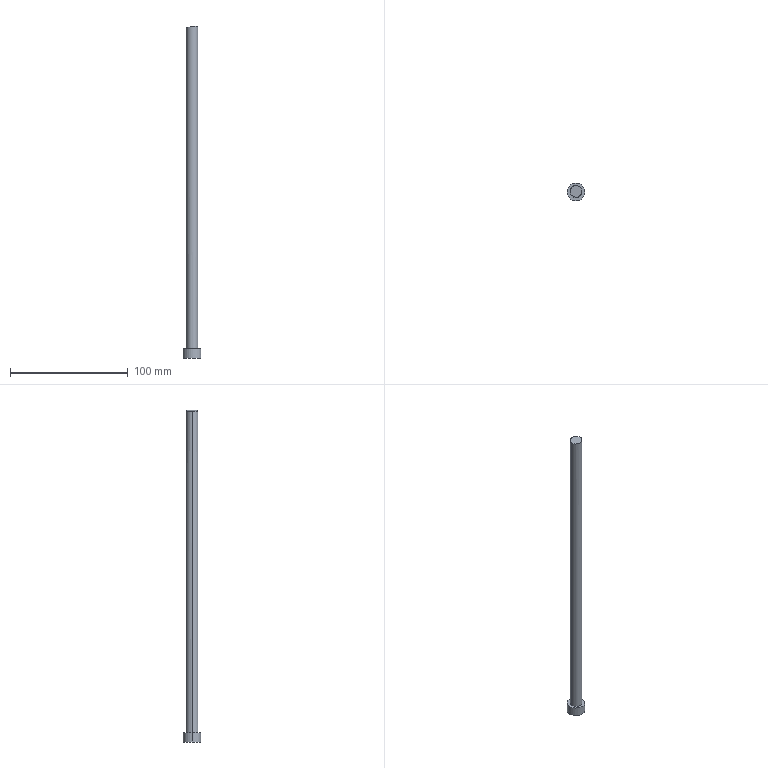Part | Creo | 1 solid | 10 faces | box 15 x 15 x 281.61 mm | volume 22797 mm3 | cylinder 6 | plane 4 | commonest cylinder face diameters 3 x2 10 x2 15 x2
STEP:
#1=CARTESIAN_POINT('',(-114.,-67.,-252.5));
#2=VERTEX_POINT('',#1);
#3=CARTESIAN_POINT('',(-124.,-67.,-252.5));
#4=VERTEX_POINT('',#3);
#5=CARTESIAN_POINT('',(-119.,-67.,-252.5));
#6=DIRECTION('',(0.,0.,-1.));
#7=DIRECTION('',(1.,0.,0.));
#8=AXIS2_PLACEMENT_3D('',#5,#6,#7);
#9=CIRCLE('',#8,5.);
#10=EDGE_CURVE('',#2,#4,#9,.T.);
#11=ORIENTED_EDGE('',*,*,#10,.T.);
#12=CARTESIAN_POINT('',(-124.,-67.,19.785));
#13=VERTEX_POINT('',#12);
#14=CARTESIAN_POINT('',(-124.,-67.,19.785));
#15=DIRECTION('',(0.,0.,-1.));
#16=VECTOR('',#15,272.285);
#17=LINE('',#14,#16);
#18=EDGE_CURVE('',#13,#4,#17,.T.);
#19=ORIENTED_EDGE('',*,*,#18,.F.);
#20=CARTESIAN_POINT('',(-114.,-67.,21.11));
#21=VERTEX_POINT('',#20);
#22=CARTESIAN_POINT('',(-124.,-67.,19.785));
#23=CARTESIAN_POINT('',(-124.,-67.589,19.785));
#24=CARTESIAN_POINT('',(-123.785,-68.862,19.813));
#25=CARTESIAN_POINT('',(-122.645,-70.641,19.964));
#26=CARTESIAN_POINT('',(-120.85,-71.786,20.202));
#27=CARTESIAN_POINT('',(-119.,-72.107,20.447));
#28=CARTESIAN_POINT('',(-117.15,-71.786,20.692));
#29=CARTESIAN_POINT('',(-115.355,-70.641,20.93));
#30=CARTESIAN_POINT('',(-114.215,-68.862,21.081));
#31=CARTESIAN_POINT('',(-114.,-67.589,21.11));
#32=CARTESIAN_POINT('',(-114.,-67.,21.11));
#33=B_SPLINE_CURVE_WITH_KNOTS('',3,(#22,#23,#24,#25,#26,#27,#28,#29,#30,#31,#32),.UNSPECIFIED.,.F.,.F.,(4,1,1,1,1,1,1,1,4),(0.,0.125,0.25,0.375,0.5,0.625,0.75,0.875,1.),.UNSPECIFIED.);
#34=EDGE_CURVE('',#13,#21,#33,.T.);
#35=ORIENTED_EDGE('',*,*,#34,.T.);
#36=CARTESIAN_POINT('',(-114.,-67.,21.11));
#37=DIRECTION('',(0.,0.,-1.));
#38=VECTOR('',#37,273.61);
#39=LINE('',#36,#38);
#40=EDGE_CURVE('',#21,#2,#39,.T.);
#41=ORIENTED_EDGE('',*,*,#40,.T.);
#42=EDGE_LOOP('',(#11,#19,#35,#41));
#43=FACE_OUTER_BOUND('',#42,.F.);
#44=CARTESIAN_POINT('',(-119.,-67.,135.));
#45=DIRECTION('',(0.,0.,-1.));
#46=DIRECTION('',(1.,0.,0.));
#47=AXIS2_PLACEMENT_3D('',#44,#45,#46);
#48=CYLINDRICAL_SURFACE('',#47,5.);
#49=ADVANCED_FACE('',(#43),#48,.T.);
#50=CARTESIAN_POINT('',(-126.5,-67.,-252.5));
#51=VERTEX_POINT('',#50);
#52=CARTESIAN_POINT('',(-111.5,-67.,-252.5));
#53=VERTEX_POINT('',#52);
#54=CARTESIAN_POINT('',(-119.,-67.,-252.5));
#55=DIRECTION('',(0.,0.,1.));
#56=DIRECTION('',(-1.,0.,0.));
#57=AXIS2_PLACEMENT_3D('',#54,#55,#56);
#58=CIRCLE('',#57,7.5);
#59=EDGE_CURVE('',#51,#53,#58,.T.);
#60=ORIENTED_EDGE('',*,*,#59,.F.);
#61=CARTESIAN_POINT('',(-119.,-67.,-252.5));
#62=DIRECTION('',(0.,0.,1.));
#63=DIRECTION('',(1.,0.,0.));
#64=AXIS2_PLACEMENT_3D('',#61,#62,#63);
#65=CIRCLE('',#64,7.5);
#66=EDGE_CURVE('',#53,#51,#65,.T.);
#67=ORIENTED_EDGE('',*,*,#66,.F.);
#68=EDGE_LOOP('',(#60,#67));
#69=FACE_OUTER_BOUND('',#68,.F.);
#70=CARTESIAN_POINT('',(-119.,-67.,-252.5));
#71=DIRECTION('',(0.,0.,-1.));
#72=DIRECTION('',(-1.,0.,0.));
#73=AXIS2_PLACEMENT_3D('',#70,#71,#72);
#74=CIRCLE('',#73,5.);
#75=EDGE_CURVE('',#4,#2,#74,.T.);
#76=ORIENTED_EDGE('',*,*,#75,.F.);
#77=ORIENTED_EDGE('',*,*,#10,.F.);
#78=EDGE_LOOP('',(#76,#77));
#79=FACE_BOUND('',#78,.F.);
#80=CARTESIAN_POINT('',(-119.,-67.,-252.5));
#81=DIRECTION('',(0.,0.,1.));
#82=DIRECTION('',(-1.,0.,0.));
#83=AXIS2_PLACEMENT_3D('',#80,#81,#82);
#84=PLANE('',#83);
#85=ADVANCED_FACE('',(#69,#79),#84,.T.);
#86=ORIENTED_EDGE('',*,*,#75,.T.);
#87=ORIENTED_EDGE('',*,*,#40,.F.);
#88=CARTESIAN_POINT('',(-114.,-67.,21.11));
#89=CARTESIAN_POINT('',(-114.,-66.411,21.11));
#90=CARTESIAN_POINT('',(-114.215,-65.138,21.081));
#91=CARTESIAN_POINT('',(-115.355,-63.359,20.93));
#92=CARTESIAN_POINT('',(-117.15,-62.214,20.692));
#93=CARTESIAN_POINT('',(-119.,-61.893,20.447));
#94=CARTESIAN_POINT('',(-120.85,-62.214,20.202));
#95=CARTESIAN_POINT('',(-122.645,-63.359,19.964));
#96=CARTESIAN_POINT('',(-123.785,-65.138,19.813));
#97=CARTESIAN_POINT('',(-124.,-66.411,19.785));
#98=CARTESIAN_POINT('',(-124.,-67.,19.785));
#99=B_SPLINE_CURVE_WITH_KNOTS('',3,(#88,#89,#90,#91,#92,#93,#94,#95,#96,#97,#98),.UNSPECIFIED.,.F.,.F.,(4,1,1,1,1,1,1,1,4),(0.,0.125,0.25,0.375,0.5,0.625,0.75,0.875,1.),.UNSPECIFIED.);
#100=EDGE_CURVE('',#21,#13,#99,.T.);
#101=ORIENTED_EDGE('',*,*,#100,.T.);
#102=ORIENTED_EDGE('',*,*,#18,.T.);
#103=EDGE_LOOP('',(#86,#87,#101,#102));
#104=FACE_OUTER_BOUND('',#103,.F.);
#105=CARTESIAN_POINT('',(-119.,-67.,135.));
#106=DIRECTION('',(0.,0.,-1.));
#107=DIRECTION('',(1.,0.,0.));
#108=AXIS2_PLACEMENT_3D('',#105,#106,#107);
#109=CYLINDRICAL_SURFACE('',#108,5.);
#110=ADVANCED_FACE('',(#104),#109,.T.);
#111=ORIENTED_EDGE('',*,*,#34,.F.);
#112=ORIENTED_EDGE('',*,*,#100,.F.);
#113=EDGE_LOOP('',(#111,#112));
#114=FACE_OUTER_BOUND('',#113,.F.);
#115=CARTESIAN_POINT('',(-129.28,-147.436,19.085));
#116=DIRECTION('',(0.1313,0.,-0.9913));
#117=DIRECTION('',(0.,-1.,0.));
#118=AXIS2_PLACEMENT_3D('',#115,#116,#117);
#119=PLANE('',#118);
#120=ADVANCED_FACE('',(#114),#119,.F.);
#121=CARTESIAN_POINT('',(-111.5,-67.,-255.));
#122=VERTEX_POINT('',#121);
#123=CARTESIAN_POINT('',(-111.5,-67.,-258.));
#124=VERTEX_POINT('',#123);
#125=CARTESIAN_POINT('',(-111.5,-67.,-255.));
#126=CARTESIAN_POINT('',(-111.5,-67.173,-255.));
#127=CARTESIAN_POINT('',(-111.512,-67.52,-255.06));
#128=CARTESIAN_POINT('',(-111.561,-67.983,-255.326));
#129=CARTESIAN_POINT('',(-111.617,-68.328,-255.738));
#130=CARTESIAN_POINT('',(-111.653,-68.508,-256.238));
#131=CARTESIAN_POINT('',(-111.653,-68.507,-256.766));
#132=CARTESIAN_POINT('',(-111.617,-68.327,-257.264));
#133=CARTESIAN_POINT('',(-111.561,-67.983,-257.674));
#134=CARTESIAN_POINT('',(-111.512,-67.52,-257.94));
#135=CARTESIAN_POINT('',(-111.5,-67.173,-258.));
#136=CARTESIAN_POINT('',(-111.5,-67.,-258.));
#137=B_SPLINE_CURVE_WITH_KNOTS('',3,(#125,#126,#127,#128,#129,#130,#131,#132,#133,#134,#135,#136),.UNSPECIFIED.,.F.,.F.,(4,1,1,1,1,1,1,1,1,4),(0.,0.1111,0.2222,0.3333,0.4444,0.5556,0.6667,0.7778,0.8889,1.),.UNSPECIFIED.);
#138=EDGE_CURVE('',#122,#124,#137,.T.);
#139=ORIENTED_EDGE('',*,*,#138,.T.);
#140=CARTESIAN_POINT('',(-111.5,-67.,-260.5));
#141=VERTEX_POINT('',#140);
#142=CARTESIAN_POINT('',(-111.5,-67.,-260.5));
#143=DIRECTION('',(-0.000006537,0.,1.));
#144=VECTOR('',#143,2.5);
#145=LINE('',#142,#144);
#146=EDGE_CURVE('',#141,#124,#145,.T.);
#147=ORIENTED_EDGE('',*,*,#146,.F.);
#148=CARTESIAN_POINT('',(-126.5,-67.,-260.5));
#149=VERTEX_POINT('',#148);
#150=CARTESIAN_POINT('',(-119.,-67.,-260.5));
#151=DIRECTION('',(0.,0.,-1.));
#152=DIRECTION('',(1.,0.,0.));
#153=AXIS2_PLACEMENT_3D('',#150,#151,#152);
#154=CIRCLE('',#153,7.5);
#155=EDGE_CURVE('',#141,#149,#154,.T.);
#156=ORIENTED_EDGE('',*,*,#155,.T.);
#157=CARTESIAN_POINT('',(-126.5,-67.,-260.5));
#158=DIRECTION('',(0.,0.,1.));
#159=VECTOR('',#158,8.);
#160=LINE('',#157,#159);
#161=EDGE_CURVE('',#149,#51,#160,.T.);
#162=ORIENTED_EDGE('',*,*,#161,.T.);
#163=ORIENTED_EDGE('',*,*,#59,.T.);
#164=CARTESIAN_POINT('',(-111.5,-67.,-255.));
#165=DIRECTION('',(0.000005048,0.,1.));
#166=VECTOR('',#165,2.5);
#167=LINE('',#164,#166);
#168=EDGE_CURVE('',#122,#53,#167,.T.);
#169=ORIENTED_EDGE('',*,*,#168,.F.);
#170=EDGE_LOOP('',(#139,#147,#156,#162,#163,#169));
#171=FACE_OUTER_BOUND('',#170,.F.);
#172=CARTESIAN_POINT('',(-119.,-67.,-260.5));
#173=DIRECTION('',(0.,0.,1.));
#174=DIRECTION('',(-1.,0.,0.));
#175=AXIS2_PLACEMENT_3D('',#172,#173,#174);
#176=CYLINDRICAL_SURFACE('',#175,7.5);
#177=ADVANCED_FACE('',(#171),#176,.T.);
#178=ORIENTED_EDGE('',*,*,#138,.F.);
#179=CARTESIAN_POINT('',(-119.,-67.,-255.));
#180=VERTEX_POINT('',#179);
#181=CARTESIAN_POINT('',(-119.,-67.,-255.));
#182=DIRECTION('',(1.,0.,-0.000004481));
#183=VECTOR('',#182,7.5);
#184=LINE('',#181,#183);
#185=EDGE_CURVE('',#180,#122,#184,.T.);
#186=ORIENTED_EDGE('',*,*,#185,.F.);
#187=CARTESIAN_POINT('',(-119.,-67.,-258.));
#188=VERTEX_POINT('',#187);
#189=CARTESIAN_POINT('',(-119.,-67.,-256.5));
#190=DIRECTION('',(1.,0.,0.));
#191=DIRECTION('',(0.,0.,1.));
#192=AXIS2_PLACEMENT_3D('',#189,#190,#191);
#193=CIRCLE('',#192,1.5);
#194=EDGE_CURVE('',#180,#188,#193,.T.);
#195=ORIENTED_EDGE('',*,*,#194,.T.);
#196=CARTESIAN_POINT('',(-119.,-67.,-258.));
#197=DIRECTION('',(1.,0.,0.000002911));
#198=VECTOR('',#197,7.5);
#199=LINE('',#196,#198);
#200=EDGE_CURVE('',#188,#124,#199,.T.);
#201=ORIENTED_EDGE('',*,*,#200,.T.);
#202=EDGE_LOOP('',(#178,#186,#195,#201));
#203=FACE_OUTER_BOUND('',#202,.F.);
#204=CARTESIAN_POINT('',(-119.,-67.,-256.5));
#205=DIRECTION('',(1.,0.,0.));
#206=DIRECTION('',(0.,0.,-1.));
#207=AXIS2_PLACEMENT_3D('',#204,#205,#206);
#208=CYLINDRICAL_SURFACE('',#207,1.5);
#209=ADVANCED_FACE('',(#203),#208,.F.);
#210=CARTESIAN_POINT('',(-111.502,-66.813,-255.012));
#211=VERTEX_POINT('',#210);
#212=CARTESIAN_POINT('',(-111.5,-67.,-255.));
#213=CARTESIAN_POINT('',(-111.5,-66.979,-255.));
#214=CARTESIAN_POINT('',(-111.5,-66.938,-255.001));
#215=CARTESIAN_POINT('',(-111.501,-66.875,-255.005));
#216=CARTESIAN_POINT('',(-111.502,-66.834,-255.009));
#217=B_SPLINE_CURVE_WITH_KNOTS('',3,(#212,#213,#214,#215,#216,#210),.UNSPECIFIED.,.F.,.F.,(4,1,1,4),(0.,0.3333,0.6667,1.),.UNSPECIFIED.);
#218=EDGE_CURVE('',#122,#211,#217,.T.);
#219=ORIENTED_EDGE('',*,*,#218,.T.);
#220=CARTESIAN_POINT('',(-111.502,-66.813,-255.012));
#221=CARTESIAN_POINT('',(-111.507,-66.616,-255.036));
#222=CARTESIAN_POINT('',(-111.531,-66.26,-255.155));
#223=CARTESIAN_POINT('',(-111.591,-65.812,-255.525));
#224=CARTESIAN_POINT('',(-111.643,-65.538,-256.03));
#225=CARTESIAN_POINT('',(-111.658,-65.467,-256.603));
#226=CARTESIAN_POINT('',(-111.628,-65.614,-257.16));
#227=CARTESIAN_POINT('',(-111.57,-65.95,-257.622));
#228=CARTESIAN_POINT('',(-111.515,-66.439,-257.928));
#229=CARTESIAN_POINT('',(-111.5,-66.803,-258.));
#230=CARTESIAN_POINT('',(-111.5,-67.,-258.));
#231=B_SPLINE_CURVE_WITH_KNOTS('',3,(#220,#221,#222,#223,#224,#225,#226,#227,#228,#229,#230),.UNSPECIFIED.,.F.,.F.,(4,1,1,1,1,1,1,1,4),(0.,0.125,0.25,0.375,0.5,0.625,0.75,0.875,1.),.UNSPECIFIED.);
#232=EDGE_CURVE('',#211,#124,#231,.T.);
#233=ORIENTED_EDGE('',*,*,#232,.T.);
#234=ORIENTED_EDGE('',*,*,#200,.F.);
#235=CARTESIAN_POINT('',(-119.,-67.,-256.5));
#236=DIRECTION('',(1.,0.,0.));
#237=DIRECTION('',(0.,0.,-1.));
#238=AXIS2_PLACEMENT_3D('',#235,#236,#237);
#239=CIRCLE('',#238,1.5);
#240=EDGE_CURVE('',#188,#180,#239,.T.);
#241=ORIENTED_EDGE('',*,*,#240,.T.);
#242=ORIENTED_EDGE('',*,*,#185,.T.);
#243=EDGE_LOOP('',(#219,#233,#234,#241,#242));
#244=FACE_OUTER_BOUND('',#243,.F.);
#245=CARTESIAN_POINT('',(-119.,-67.,-256.5));
#246=DIRECTION('',(1.,0.,0.));
#247=DIRECTION('',(0.,0.,-1.));
#248=AXIS2_PLACEMENT_3D('',#245,#246,#247);
#249=CYLINDRICAL_SURFACE('',#248,1.5);
#250=ADVANCED_FACE('',(#244),#249,.F.);
#251=ORIENTED_EDGE('',*,*,#232,.F.);
#252=ORIENTED_EDGE('',*,*,#218,.F.);
#253=ORIENTED_EDGE('',*,*,#168,.T.);
#254=ORIENTED_EDGE('',*,*,#66,.T.);
#255=ORIENTED_EDGE('',*,*,#161,.F.);
#256=CARTESIAN_POINT('',(-119.,-67.,-260.5));
#257=DIRECTION('',(0.,0.,-1.));
#258=DIRECTION('',(-1.,0.,0.));
#259=AXIS2_PLACEMENT_3D('',#256,#257,#258);
#260=CIRCLE('',#259,7.5);
#261=EDGE_CURVE('',#149,#141,#260,.T.);
#262=ORIENTED_EDGE('',*,*,#261,.T.);
#263=ORIENTED_EDGE('',*,*,#146,.T.);
#264=EDGE_LOOP('',(#251,#252,#253,#254,#255,#262,#263));
#265=FACE_OUTER_BOUND('',#264,.F.);
#266=CARTESIAN_POINT('',(-119.,-67.,-260.5));
#267=DIRECTION('',(0.,0.,1.));
#268=DIRECTION('',(-1.,0.,0.));
#269=AXIS2_PLACEMENT_3D('',#266,#267,#268);
#270=CYLINDRICAL_SURFACE('',#269,7.5);
#271=ADVANCED_FACE('',(#265),#270,.T.);
#272=ORIENTED_EDGE('',*,*,#155,.F.);
#273=ORIENTED_EDGE('',*,*,#261,.F.);
#274=EDGE_LOOP('',(#272,#273));
#275=FACE_OUTER_BOUND('',#274,.F.);
#276=CARTESIAN_POINT('',(143.714,75.015,-260.5));
#277=DIRECTION('',(0.,0.,-1.));
#278=DIRECTION('',(1.,0.,0.));
#279=AXIS2_PLACEMENT_3D('',#276,#277,#278);
#280=PLANE('',#279);
#281=ADVANCED_FACE('',(#275),#280,.T.);
#282=ORIENTED_EDGE('',*,*,#240,.F.);
#283=ORIENTED_EDGE('',*,*,#194,.F.);
#284=EDGE_LOOP('',(#282,#283));
#285=FACE_OUTER_BOUND('',#284,.F.);
#286=CARTESIAN_POINT('',(-119.,-67.,-256.5));
#287=DIRECTION('',(-1.,0.,0.));
#288=DIRECTION('',(0.,0.,1.));
#289=AXIS2_PLACEMENT_3D('',#286,#287,#288);
#290=PLANE('',#289);
#291=ADVANCED_FACE('',(#285),#290,.F.);
#292=CLOSED_SHELL('',(#49,#85,#110,#120,#177,#209,#250,#271,#281,#291));
#293=MANIFOLD_SOLID_BREP('',#292);
#294=(LENGTH_UNIT()NAMED_UNIT(*)SI_UNIT(.MILLI.,.METRE.));
#295=UNCERTAINTY_MEASURE_WITH_UNIT(LENGTH_MEASURE(0.02824),#294,'','');
#296=(NAMED_UNIT(*)PLANE_ANGLE_UNIT()SI_UNIT($,.RADIAN.));
#297=PLANE_ANGLE_MEASURE_WITH_UNIT(PLANE_ANGLE_MEASURE(0.01745),#296);
#298=(CONVERSION_BASED_UNIT('DEGREE',#297)NAMED_UNIT(*)PLANE_ANGLE_UNIT());
#299=(NAMED_UNIT(*)SI_UNIT($,.STERADIAN.)SOLID_ANGLE_UNIT());
#300=(GEOMETRIC_REPRESENTATION_CONTEXT(3)GLOBAL_UNCERTAINTY_ASSIGNED_CONTEXT((#295))GLOBAL_UNIT_ASSIGNED_CONTEXT((#294,#298,#299))REPRESENTATION_CONTEXT('',''));
#301=ADVANCED_BREP_SHAPE_REPRESENTATION('',(#293),#300);